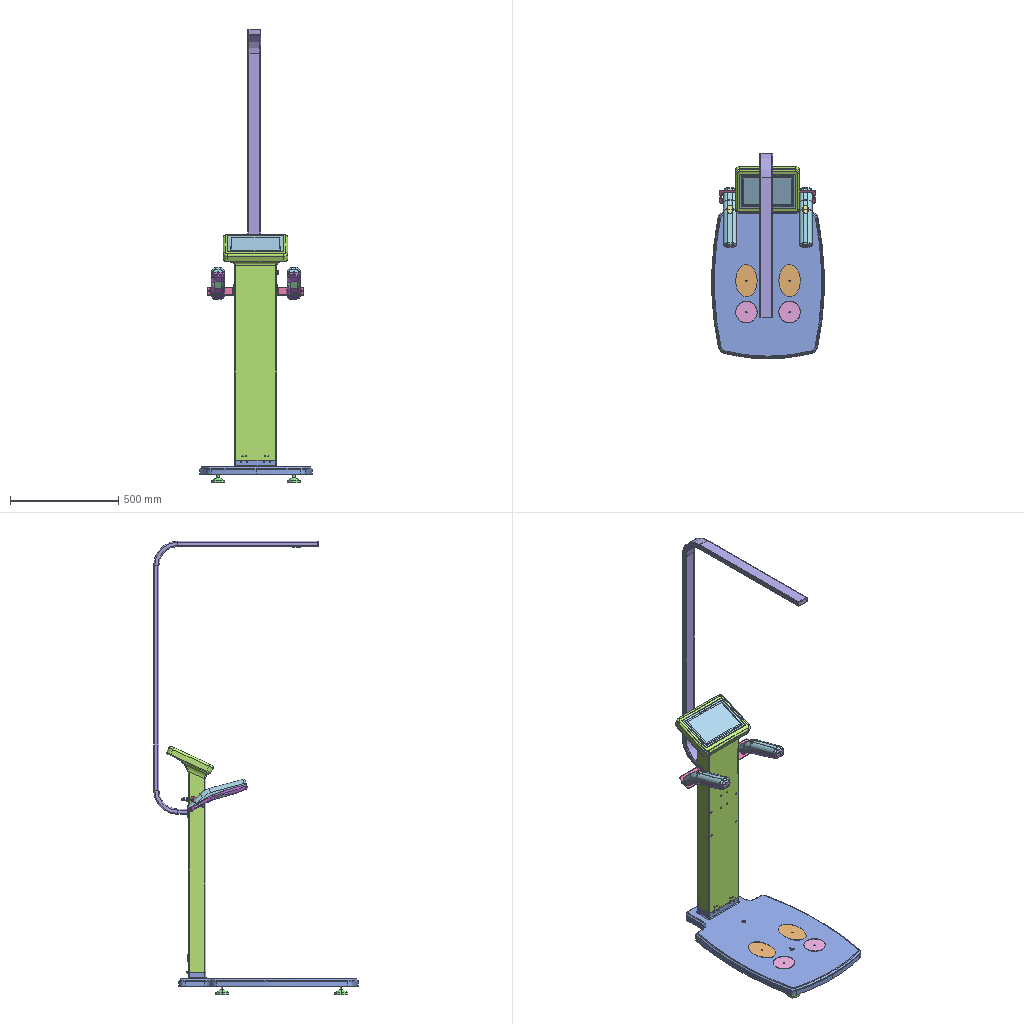Assembly | SolidWorks | 34 different items | 59 placed | box 519 x 948 x 2100 mm
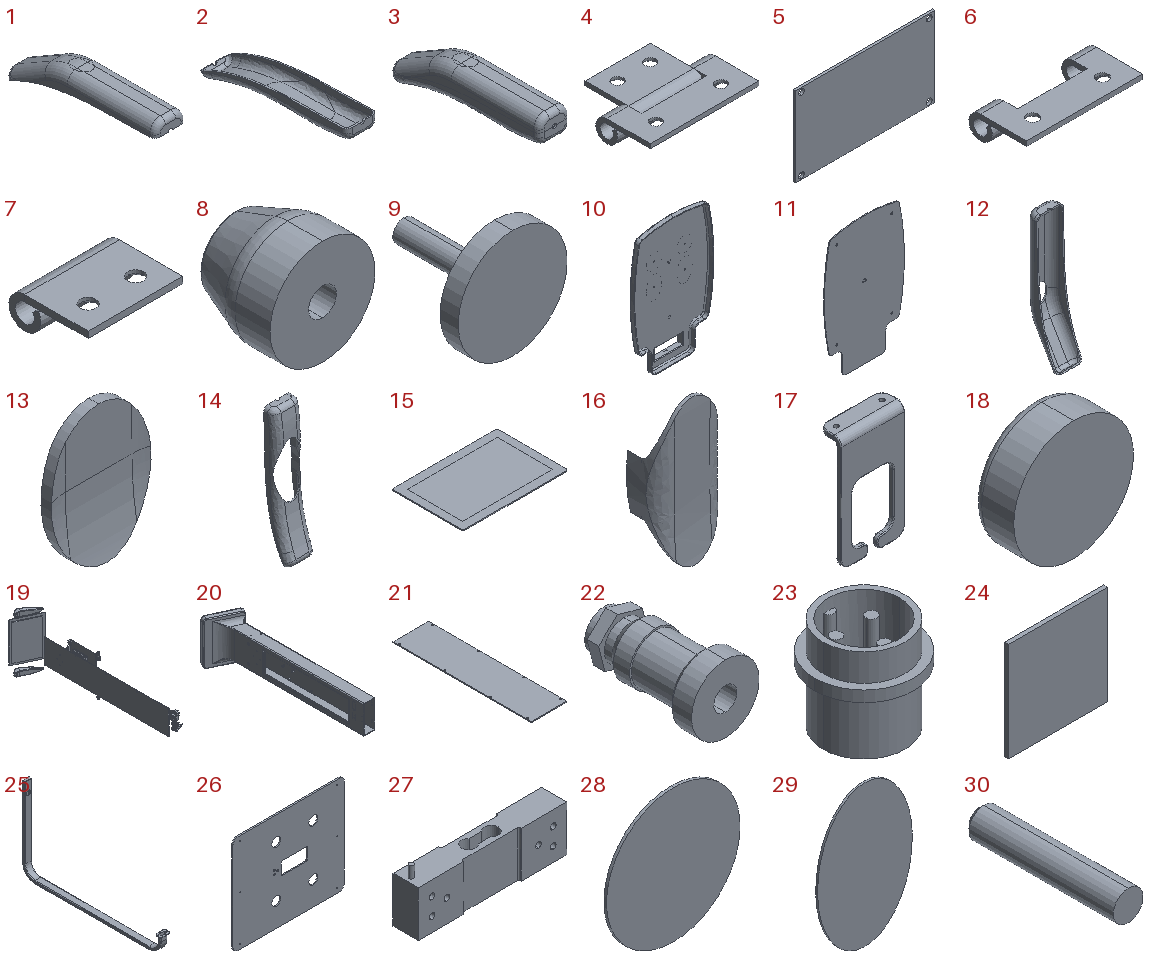Parts list (item | name | quantity | parent item | size | volume | features):
1 | (subassembly) | x2 | in 3 | 60 x 290.622 x 70.555 mm | 84963 mm3 | -
2 | (subassembly) | x2 | in 3 | 60 x 286.282 x 56.047 mm | 79320 mm3 | features CompositeCurve 2
3 | (subassembly) | x2 | - | 60 x 290.622 x 81.047 mm | 164282 mm3 | -
4 | (subassembly) | x3 | - | 50 x 40 x 10 mm | 4742 mm3 | -
5 | - | x1 | - | 73.3 x 1.5 x 42 mm | 4575 mm3 | features FlatPattern 1, SMBaseFlange 1, SheetMetal 1
6 | - | x3 | in 4 | 50 x 25 x 10 mm | 2381 mm3 | features ICE 2, Chamfer 1, FlatPattern 1, SMBaseFlange 1, SheetMetal 1
7 | - | x3 | in 4 | 30 x 25 x 10 mm | 2360 mm3 | features Chamfer 1, FlatPattern 1, ICE 1, SMBaseFlange 1, SheetMetal 1
8 | - | x1 | - | 30 x 25 x 30 mm | 12754 mm3 | features Revolution 1
9 | - | x4 | - | 60 x 60 x 60 mm | 49763 mm3 | features Revolution 1
10 | - | x1 | - | 521.263 x 65 x 830.32 mm | 2069841 mm3 | features ICE 6, Cut 4, Fillet 3, Chamfer 2, Extrusion 1, Shell 1
11 | - | x1 | - | 509.263 x 5 x 818.32 mm | 1799381 mm3 | features ICE 4, Fillet 2, Chamfer 1, Cut 1, Extrusion 1
12 | - | x2 | in 1 | 60 x 70.555 x 290.622 mm | 82120 mm3 | features ICE 5, Fillet 4, Extrusion 1, Shell 1
13 | - | x2 | in 1 | 30 x 5.528 x 40 mm | 2843 mm3 | features ICE 5, Fillet 4, Extrusion 1, Shell 1
14 | - | x2 | in 2 | 60 x 56.047 x 286.282 mm | 59965 mm3 | features ICE 5, Fillet 4, Extrusion 1, Shell 1
15 | - | x1 | - | 256.55 x 174.5 x 7.5 mm | 282503 mm3 | features ICE 2, Extrusion 1
16 | - | x2 | in 2 | 58 x 29.373 x 120 mm | 19355 mm3 | features ICE 5, Fillet 4, Extrusion 1, Shell 1
17 | - | x2 | - | 70 x 25 x 125 mm | 34149 mm3 | features Fillet 3, ICE 2, FlatPattern 1, SMBaseFlange 1, SheetMetal 1
18 | - | x1 | - | 15 x 5 x 15 mm | 856.761 mm3 | features Fillet 1, FlatPattern 1, ICE 1, SMBaseFlange 1, SheetMetal 1
19 | - | x1 | - | 159.207 x 1008 x 361.7 mm | 990994 mm3 | features BaseBody 22, Fillet 2, ICE 2, Cut 1
20 | - | x1 | - | 215.89 x 1045 x 300 mm | 2133563 mm3 | features ICE 21, Fillet 9, Cut 4, MirrorPattern 2, Extrusion 1, HoleWzd 1, Shell 1
21 | - | x1 | - | 155 x 600 x 4 mm | 371585 mm3 | features Extrusion 1, HoleWzd 1, ICE 1
22 | - | x2 | - | 17.4 x 31.2 x 17.4 mm | 3464 mm3 | features ICE 2, Chamfer 1, Revolution 1
23 | - | x2 | - | 18 x 18 x 17 mm | 1920 mm3 | features ICE 4, Extrusion 1
24 | - | x1 | - | 50 x 7 x 50 mm | 10765 mm3 | features Fillet 1, FlatPattern 1, ICE 1, SMBaseFlange 1, SheetMetal 1
25 | - | x1 | - | 90 x 1280 x 762.5 mm | 652548 mm3 | features ICE 4, Fillet 2, Sweep 1
26 | - | x1 | - | 435 x 4 x 385 mm | 632168 mm3 | features Cut 4, Extrusion 1, Fillet 1, HoleWzd 1
27 | - | x1 | - | 130 x 22 x 50 mm | 92053 mm3 | features ICE 3, Extrusion 1, Fillet 1, HoleWzd 1
28 | - | x2 | - | 100 x 2 x 100 mm | 15708 mm3 | features Extrusion 1
29 | - | x2 | - | 100 x 2 x 150 mm | 23563 mm3 | features Extrusion 1
30 | - | x4 | - | 3 x 15 x 3 mm | 104.982 mm3 | features Chamfer 1, Extrusion 1
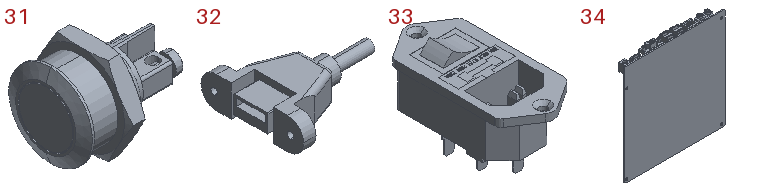31 | - | x1 | - | 24.5 x 21.8 x 18.879 mm | 3360 mm3 | features ICE 13, Chamfer 5, Revolution 5, Fillet 4
32 | - | x2 | - | 44.9 x 39 x 12 mm | 5891 mm3 | features Fillet 3, ICE 3, Extrusion 1, HoleWzd 1
33 | - | x1 | - | 30.8 x 65.077 x 35.364 mm | 20568 mm3 | features ICE 17, Chamfer 3, Fillet 3, Extrusion 1, HoleWzd 1
34 | - | x1 | - | 170 x 17.2 x 176.85 mm | 110739 mm3 | features ICE 21, Fillet 3, Chamfer 2, Extrusion 1, HoleWzd 1
Mates (type | each side: item.copy, entity, surface, feature):
In the top assembly
Coincident | 10.1 face plane Boss-Extrude1 | 11.1 face plane Boss-Extrude1
Parallel | 11.1 face plane Cut-Extrude4 | 10.1 face plane Boss-Extrude1 | 2 times
Coincident | 10.1 face plane Boss-Extrude3 | 20.1 face plane Boss-Extrude2 | 2 times
DistanceDim | 11.1 face plane Boss-Extrude1 | 28.1 face plane Boss-Extrude1
Concentric | 28.1 face cylinder Boss-Extrude1 | 30.1 face cylinder Boss-Extrude1
Coincident | 28.1 face plane Boss-Extrude1 | 30.1 face plane Boss-Extrude1
Coincident | 28.1 face plane Boss-Extrude1 | 29.1 face plane Boss-Extrude1
DistanceDim | 29.1 plane | 28.1 face cylinder Boss-Extrude1
Coincident | 30.1 face plane Boss-Extrude1 | 30.2 face plane Boss-Extrude1
Concentric | 11.1 face cylinder Cut-Extrude1 | 9.1 face cylinder Revolve1
DistanceDim | 9.1 face plane Revolve1 | 11.1 face plane Boss-Extrude1
Coincident | 20.1 face plane Boss-Extrude17 | 34.1 face plane Boss-Extrude1
Concentric | 20.1 face cylinder Boss-Extrude17 | 34.1 face cylinder Cut-Extrude1
Parallel | 20.1 face plane Shell1 | 34.1 face plane Boss-Extrude1
Coincident | 20.1 face plane Boss-Extrude1 | 15.1 face plane Boss-Extrude1
Coincident | 20.1 face plane Cut-Extrude1 | 15.1 face plane Boss-Extrude1 | 2 times
Coincident | 20.1 face plane Boss-Extrude18 | 5.1 face plane Base-Flange1
Concentric | 20.1 face cylinder Boss-Extrude18 | 5.1 face cylinder Base-Flange1 | 2 times
Coincident | 20.1 face plane Boss-Extrude2 | 21.1 face plane Boss-Extrude1
Concentric | 20.1 face cylinder M3 Tapped Hole1 | 21.1 face cylinder Hole Size Slotted Countersunk Head Screw Type1 | 2 times
Coincident | 20.1 face plane Boss-Extrude2 | 31.1 face plane Revolve2
Concentric | 20.1 face cylinder Cut-Extrude13 | 31.1 face cylinder Revolve1
Concentric | 20.1 face cylinder Cut-Extrude17 | 23.1 face cylinder Boss-Extrude2
Coincident | 20.1 face plane Boss-Extrude2 | 23.1 face plane Boss-Extrude1
Coincident | 20.1 face plane Boss-Extrude2 | 33.1 face plane Boss-Extrude1
Coincident | 20.1 face plane Cut-Extrude10 | 33.1 face plane Boss-Extrude2 | 2 times
Concentric | 20.1 face cylinder Cut-Extrude12 | 32.1 face cylinder M3 Tapped Hole1
Concentric | 32.1 face cylinder M3 Tapped Hole1 | 20.1 face cylinder Cut-Extrude12
Coincident | 20.1 edge | 32.1 face plane Boss-Extrude1
Concentric | 23.1 face cylinder Boss-Extrude2 | 22.1 face cylinder Revolve1
Coincident | 23.1 face plane Boss-Extrude1 | 22.1 edge
Coincident | 10.1 face plane Boss-Extrude3 | 20.1 face plane Cut-Extrude6
Coincident | 10.1 face plane Boss-Extrude3 | 6.1 face plane Base-Flange1
DistanceDim | 6.1 face cylinder Base Bend1 | 10.1 face plane Boss-Extrude3
DistanceDim | 6.1 face plane Base Bend1 | 10.1 face plane Boss-Extrude3
Concentric | 10.1 face cylinder Cut-Extrude5 | 18.1 face cylinder Base-Flange1
DistanceDim | 18.1 face plane Base-Flange1 | 10.1 face plane Boss-Extrude1
Coincident | 20.1 face plane Boss-Extrude2 | 6.2 face plane Base-Flange1
Coincident | 20.1 edge | 6.2 edge
Coincident | 20.1 face plane Boss-Extrude2 | 25.1 face plane Sweep-Thin Part2
DistanceDim | 20.1 face plane Boss-Extrude2 | 25.1 face plane Boss-Extrude2
DistanceDim | 10.1 face plane Boss-Extrude1 | 25.1 face plane Sweep-Thin Part2
Coincident | 25.1 edge | 24.1 face plane Base-Flange1
Concentric | 25.1 face cylinder Cut-Extrude2 | 24.1 face cylinder Boss-Extrude1
Coincident | 20.1 face plane Boss-Extrude2 | 17.1 face plane Base-Flange1
DistanceDim | 20.1 face plane Boss-Extrude2 | 17.1 face cylinder Cut-Extrude2
PlanarAngleDim | 12.1 face plane Boss-Extrude1 | 17.1 face plane Base-Flange1
PlanarAngleDim | 17.1 face plane Base-Flange1 | 20.1 face plane Boss-Extrude2
DistanceDim | 12.1 face plane Boss-Extrude1 | 17.1 face plane Cut-Extrude1
Coincident | 20.1 face plane Boss-Extrude2 | 17.2 face plane Base-Flange1
DistanceDim | 20.1 face plane Boss-Extrude2 | 17.2 face cylinder Cut-Extrude2
Coincident | 17.1 face plane Base-Flange1 | 17.2 face plane Base-Flange1
In subassembly 4
Concentric | 6.3 face cylinder Base Bend1 | 7.1 face cylinder Base Bend1
Coincident | 6.3 face plane Cut-Extrude1 | 7.1 face plane Base-Flange1
Coincident | 6.3 face plane Base-Flange1 | 7.1 face plane Base-Flange1
In subassembly 3
Coincident | 12.2 plane | 14.1 plane | 3 times
In subassembly 1
Coincident | 12.3 plane | 13.1 plane | 3 times
In subassembly 2
Coincident | 14.2 plane | 16.1 plane | 3 times